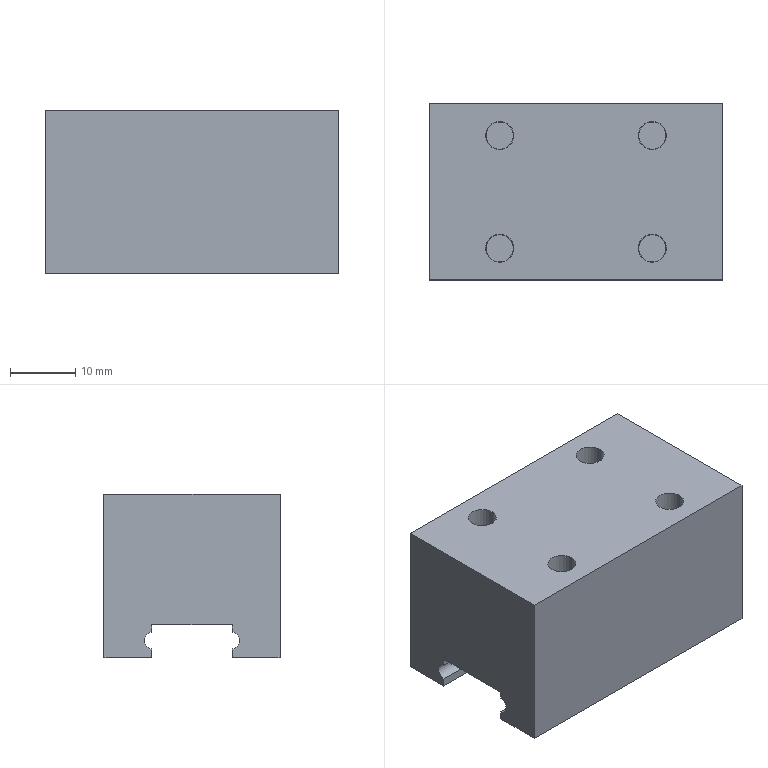Part | SolidWorks | features BaseBody 1 | 1 solid | 38 faces | box 45 x 27 x 25 mm | volume 26500 mm3 | plane 20 | cylinder 18 | commonest cylinder face diameters 4.2 x8 4.3 x8 2.6 x2
STEP:
#1=CARTESIAN_POINT('',(9.55,8.64,21.8));
#2=VERTEX_POINT('',#1);
#3=CARTESIAN_POINT('',(13.85,8.64,21.8));
#4=VERTEX_POINT('',#3);
#5=CARTESIAN_POINT('',(11.7,8.64,21.8));
#6=DIRECTION('',(0.,0.,1.));
#7=DIRECTION('',(1.,0.,0.));
#8=AXIS2_PLACEMENT_3D('',#5,#6,#7);
#9=CIRCLE('',#8,2.15);
#10=EDGE_CURVE('',#2,#4,#9,.T.);
#11=ORIENTED_EDGE('',*,*,#10,.F.);
#12=CARTESIAN_POINT('',(9.55,8.64,28.));
#13=VERTEX_POINT('',#12);
#14=CARTESIAN_POINT('',(9.55,8.64,21.8));
#15=DIRECTION('',(0.,0.,1.));
#16=VECTOR('',#15,1000.);
#17=LINE('',#14,#16);
#18=EDGE_CURVE('',#2,#13,#17,.T.);
#19=ORIENTED_EDGE('',*,*,#18,.T.);
#20=CARTESIAN_POINT('',(13.85,8.64,28.));
#21=VERTEX_POINT('',#20);
#22=CARTESIAN_POINT('',(11.7,8.64,28.));
#23=DIRECTION('',(0.,0.,-1.));
#24=DIRECTION('',(1.,0.,0.));
#25=AXIS2_PLACEMENT_3D('',#22,#23,#24);
#26=CIRCLE('',#25,2.15);
#27=EDGE_CURVE('',#21,#13,#26,.T.);
#28=ORIENTED_EDGE('',*,*,#27,.F.);
#29=CARTESIAN_POINT('',(13.85,8.64,21.8));
#30=DIRECTION('',(0.,0.,1.));
#31=VECTOR('',#30,1000.);
#32=LINE('',#29,#31);
#33=EDGE_CURVE('',#4,#21,#32,.T.);
#34=ORIENTED_EDGE('',*,*,#33,.F.);
#35=EDGE_LOOP('',(#11,#19,#28,#34));
#36=FACE_OUTER_BOUND('',#35,.T.);
#37=CARTESIAN_POINT('',(11.7,8.64,21.8));
#38=DIRECTION('',(0.,0.,1.));
#39=DIRECTION('',(1.,0.,0.));
#40=AXIS2_PLACEMENT_3D('',#37,#38,#39);
#41=CYLINDRICAL_SURFACE('',#40,2.15);
#42=ADVANCED_FACE('',(#36),#41,.F.);
#43=CARTESIAN_POINT('',(-13.85,8.64,21.8));
#44=VERTEX_POINT('',#43);
#45=CARTESIAN_POINT('',(-9.55,8.64,21.8));
#46=VERTEX_POINT('',#45);
#47=CARTESIAN_POINT('',(-11.7,8.64,21.8));
#48=DIRECTION('',(0.,0.,1.));
#49=DIRECTION('',(1.,0.,0.));
#50=AXIS2_PLACEMENT_3D('',#47,#48,#49);
#51=CIRCLE('',#50,2.15);
#52=EDGE_CURVE('',#44,#46,#51,.T.);
#53=ORIENTED_EDGE('',*,*,#52,.F.);
#54=CARTESIAN_POINT('',(-13.85,8.64,28.));
#55=VERTEX_POINT('',#54);
#56=CARTESIAN_POINT('',(-13.85,8.64,21.8));
#57=DIRECTION('',(0.,0.,1.));
#58=VECTOR('',#57,1000.);
#59=LINE('',#56,#58);
#60=EDGE_CURVE('',#44,#55,#59,.T.);
#61=ORIENTED_EDGE('',*,*,#60,.T.);
#62=CARTESIAN_POINT('',(-9.55,8.64,28.));
#63=VERTEX_POINT('',#62);
#64=CARTESIAN_POINT('',(-11.7,8.64,28.));
#65=DIRECTION('',(0.,0.,-1.));
#66=DIRECTION('',(1.,0.,0.));
#67=AXIS2_PLACEMENT_3D('',#64,#65,#66);
#68=CIRCLE('',#67,2.15);
#69=EDGE_CURVE('',#63,#55,#68,.T.);
#70=ORIENTED_EDGE('',*,*,#69,.F.);
#71=CARTESIAN_POINT('',(-9.55,8.64,21.8));
#72=DIRECTION('',(0.,0.,1.));
#73=VECTOR('',#72,1000.);
#74=LINE('',#71,#73);
#75=EDGE_CURVE('',#46,#63,#74,.T.);
#76=ORIENTED_EDGE('',*,*,#75,.F.);
#77=EDGE_LOOP('',(#53,#61,#70,#76));
#78=FACE_OUTER_BOUND('',#77,.T.);
#79=CARTESIAN_POINT('',(-11.7,8.64,21.8));
#80=DIRECTION('',(0.,0.,1.));
#81=DIRECTION('',(1.,0.,0.));
#82=AXIS2_PLACEMENT_3D('',#79,#80,#81);
#83=CYLINDRICAL_SURFACE('',#82,2.15);
#84=ADVANCED_FACE('',(#78),#83,.F.);
#85=CARTESIAN_POINT('',(9.55,-8.64,21.8));
#86=VERTEX_POINT('',#85);
#87=CARTESIAN_POINT('',(13.85,-8.64,21.8));
#88=VERTEX_POINT('',#87);
#89=CARTESIAN_POINT('',(11.7,-8.64,21.8));
#90=DIRECTION('',(0.,0.,1.));
#91=DIRECTION('',(1.,0.,0.));
#92=AXIS2_PLACEMENT_3D('',#89,#90,#91);
#93=CIRCLE('',#92,2.15);
#94=EDGE_CURVE('',#86,#88,#93,.T.);
#95=ORIENTED_EDGE('',*,*,#94,.F.);
#96=CARTESIAN_POINT('',(9.55,-8.64,28.));
#97=VERTEX_POINT('',#96);
#98=CARTESIAN_POINT('',(9.55,-8.64,21.8));
#99=DIRECTION('',(0.,0.,1.));
#100=VECTOR('',#99,1000.);
#101=LINE('',#98,#100);
#102=EDGE_CURVE('',#86,#97,#101,.T.);
#103=ORIENTED_EDGE('',*,*,#102,.T.);
#104=CARTESIAN_POINT('',(13.85,-8.64,28.));
#105=VERTEX_POINT('',#104);
#106=CARTESIAN_POINT('',(11.7,-8.64,28.));
#107=DIRECTION('',(0.,0.,-1.));
#108=DIRECTION('',(1.,0.,0.));
#109=AXIS2_PLACEMENT_3D('',#106,#107,#108);
#110=CIRCLE('',#109,2.15);
#111=EDGE_CURVE('',#105,#97,#110,.T.);
#112=ORIENTED_EDGE('',*,*,#111,.F.);
#113=CARTESIAN_POINT('',(13.85,-8.64,21.8));
#114=DIRECTION('',(0.,0.,1.));
#115=VECTOR('',#114,1000.);
#116=LINE('',#113,#115);
#117=EDGE_CURVE('',#88,#105,#116,.T.);
#118=ORIENTED_EDGE('',*,*,#117,.F.);
#119=EDGE_LOOP('',(#95,#103,#112,#118));
#120=FACE_OUTER_BOUND('',#119,.T.);
#121=CARTESIAN_POINT('',(11.7,-8.64,21.8));
#122=DIRECTION('',(0.,0.,1.));
#123=DIRECTION('',(1.,0.,0.));
#124=AXIS2_PLACEMENT_3D('',#121,#122,#123);
#125=CYLINDRICAL_SURFACE('',#124,2.15);
#126=ADVANCED_FACE('',(#120),#125,.F.);
#127=CARTESIAN_POINT('',(-13.85,-8.64,21.8));
#128=VERTEX_POINT('',#127);
#129=CARTESIAN_POINT('',(-9.55,-8.64,21.8));
#130=VERTEX_POINT('',#129);
#131=CARTESIAN_POINT('',(-11.7,-8.64,21.8));
#132=DIRECTION('',(0.,0.,1.));
#133=DIRECTION('',(1.,0.,0.));
#134=AXIS2_PLACEMENT_3D('',#131,#132,#133);
#135=CIRCLE('',#134,2.15);
#136=EDGE_CURVE('',#128,#130,#135,.T.);
#137=ORIENTED_EDGE('',*,*,#136,.F.);
#138=CARTESIAN_POINT('',(-13.85,-8.64,28.));
#139=VERTEX_POINT('',#138);
#140=CARTESIAN_POINT('',(-13.85,-8.64,21.8));
#141=DIRECTION('',(0.,0.,1.));
#142=VECTOR('',#141,1000.);
#143=LINE('',#140,#142);
#144=EDGE_CURVE('',#128,#139,#143,.T.);
#145=ORIENTED_EDGE('',*,*,#144,.T.);
#146=CARTESIAN_POINT('',(-9.55,-8.64,28.));
#147=VERTEX_POINT('',#146);
#148=CARTESIAN_POINT('',(-11.7,-8.64,28.));
#149=DIRECTION('',(0.,0.,-1.));
#150=DIRECTION('',(1.,0.,0.));
#151=AXIS2_PLACEMENT_3D('',#148,#149,#150);
#152=CIRCLE('',#151,2.15);
#153=EDGE_CURVE('',#147,#139,#152,.T.);
#154=ORIENTED_EDGE('',*,*,#153,.F.);
#155=CARTESIAN_POINT('',(-9.55,-8.64,21.8));
#156=DIRECTION('',(0.,0.,1.));
#157=VECTOR('',#156,1000.);
#158=LINE('',#155,#157);
#159=EDGE_CURVE('',#130,#147,#158,.T.);
#160=ORIENTED_EDGE('',*,*,#159,.F.);
#161=EDGE_LOOP('',(#137,#145,#154,#160));
#162=FACE_OUTER_BOUND('',#161,.T.);
#163=CARTESIAN_POINT('',(-11.7,-8.64,21.8));
#164=DIRECTION('',(0.,0.,1.));
#165=DIRECTION('',(1.,0.,0.));
#166=AXIS2_PLACEMENT_3D('',#163,#164,#165);
#167=CYLINDRICAL_SURFACE('',#166,2.15);
#168=ADVANCED_FACE('',(#162),#167,.F.);
#169=CARTESIAN_POINT('',(9.6,8.64,12.));
#170=VERTEX_POINT('',#169);
#171=CARTESIAN_POINT('',(13.8,8.64,12.));
#172=VERTEX_POINT('',#171);
#173=CARTESIAN_POINT('',(11.7,8.64,12.));
#174=DIRECTION('',(0.,0.,1.));
#175=DIRECTION('',(1.,0.,0.));
#176=AXIS2_PLACEMENT_3D('',#173,#174,#175);
#177=CIRCLE('',#176,2.1);
#178=EDGE_CURVE('',#170,#172,#177,.T.);
#179=ORIENTED_EDGE('',*,*,#178,.F.);
#180=CARTESIAN_POINT('',(9.6,8.64,21.8));
#181=VERTEX_POINT('',#180);
#182=CARTESIAN_POINT('',(9.6,8.64,12.));
#183=DIRECTION('',(0.,0.,1.));
#184=VECTOR('',#183,1000.);
#185=LINE('',#182,#184);
#186=EDGE_CURVE('',#170,#181,#185,.T.);
#187=ORIENTED_EDGE('',*,*,#186,.T.);
#188=CARTESIAN_POINT('',(13.8,8.64,21.8));
#189=VERTEX_POINT('',#188);
#190=CARTESIAN_POINT('',(11.7,8.64,21.8));
#191=DIRECTION('',(0.,0.,-1.));
#192=DIRECTION('',(1.,0.,0.));
#193=AXIS2_PLACEMENT_3D('',#190,#191,#192);
#194=CIRCLE('',#193,2.1);
#195=EDGE_CURVE('',#189,#181,#194,.T.);
#196=ORIENTED_EDGE('',*,*,#195,.F.);
#197=CARTESIAN_POINT('',(13.8,8.64,12.));
#198=DIRECTION('',(0.,0.,1.));
#199=VECTOR('',#198,1000.);
#200=LINE('',#197,#199);
#201=EDGE_CURVE('',#172,#189,#200,.T.);
#202=ORIENTED_EDGE('',*,*,#201,.F.);
#203=EDGE_LOOP('',(#179,#187,#196,#202));
#204=FACE_OUTER_BOUND('',#203,.T.);
#205=CARTESIAN_POINT('',(11.7,8.64,12.));
#206=DIRECTION('',(0.,0.,1.));
#207=DIRECTION('',(1.,0.,0.));
#208=AXIS2_PLACEMENT_3D('',#205,#206,#207);
#209=CYLINDRICAL_SURFACE('',#208,2.1);
#210=ADVANCED_FACE('',(#204),#209,.F.);
#211=CARTESIAN_POINT('',(-13.8,8.64,12.));
#212=VERTEX_POINT('',#211);
#213=CARTESIAN_POINT('',(-9.6,8.64,12.));
#214=VERTEX_POINT('',#213);
#215=CARTESIAN_POINT('',(-11.7,8.64,12.));
#216=DIRECTION('',(0.,0.,1.));
#217=DIRECTION('',(1.,0.,0.));
#218=AXIS2_PLACEMENT_3D('',#215,#216,#217);
#219=CIRCLE('',#218,2.1);
#220=EDGE_CURVE('',#212,#214,#219,.T.);
#221=ORIENTED_EDGE('',*,*,#220,.F.);
#222=CARTESIAN_POINT('',(-13.8,8.64,21.8));
#223=VERTEX_POINT('',#222);
#224=CARTESIAN_POINT('',(-13.8,8.64,12.));
#225=DIRECTION('',(0.,0.,1.));
#226=VECTOR('',#225,1000.);
#227=LINE('',#224,#226);
#228=EDGE_CURVE('',#212,#223,#227,.T.);
#229=ORIENTED_EDGE('',*,*,#228,.T.);
#230=CARTESIAN_POINT('',(-9.6,8.64,21.8));
#231=VERTEX_POINT('',#230);
#232=CARTESIAN_POINT('',(-11.7,8.64,21.8));
#233=DIRECTION('',(0.,0.,-1.));
#234=DIRECTION('',(1.,0.,0.));
#235=AXIS2_PLACEMENT_3D('',#232,#233,#234);
#236=CIRCLE('',#235,2.1);
#237=EDGE_CURVE('',#231,#223,#236,.T.);
#238=ORIENTED_EDGE('',*,*,#237,.F.);
#239=CARTESIAN_POINT('',(-9.6,8.64,12.));
#240=DIRECTION('',(0.,0.,1.));
#241=VECTOR('',#240,1000.);
#242=LINE('',#239,#241);
#243=EDGE_CURVE('',#214,#231,#242,.T.);
#244=ORIENTED_EDGE('',*,*,#243,.F.);
#245=EDGE_LOOP('',(#221,#229,#238,#244));
#246=FACE_OUTER_BOUND('',#245,.T.);
#247=CARTESIAN_POINT('',(-11.7,8.64,12.));
#248=DIRECTION('',(0.,0.,1.));
#249=DIRECTION('',(1.,0.,0.));
#250=AXIS2_PLACEMENT_3D('',#247,#248,#249);
#251=CYLINDRICAL_SURFACE('',#250,2.1);
#252=ADVANCED_FACE('',(#246),#251,.F.);
#253=CARTESIAN_POINT('',(9.6,-8.64,12.));
#254=VERTEX_POINT('',#253);
#255=CARTESIAN_POINT('',(13.8,-8.64,12.));
#256=VERTEX_POINT('',#255);
#257=CARTESIAN_POINT('',(11.7,-8.64,12.));
#258=DIRECTION('',(0.,0.,1.));
#259=DIRECTION('',(1.,0.,0.));
#260=AXIS2_PLACEMENT_3D('',#257,#258,#259);
#261=CIRCLE('',#260,2.1);
#262=EDGE_CURVE('',#254,#256,#261,.T.);
#263=ORIENTED_EDGE('',*,*,#262,.F.);
#264=CARTESIAN_POINT('',(9.6,-8.64,21.8));
#265=VERTEX_POINT('',#264);
#266=CARTESIAN_POINT('',(9.6,-8.64,12.));
#267=DIRECTION('',(0.,0.,1.));
#268=VECTOR('',#267,1000.);
#269=LINE('',#266,#268);
#270=EDGE_CURVE('',#254,#265,#269,.T.);
#271=ORIENTED_EDGE('',*,*,#270,.T.);
#272=CARTESIAN_POINT('',(13.8,-8.64,21.8));
#273=VERTEX_POINT('',#272);
#274=CARTESIAN_POINT('',(11.7,-8.64,21.8));
#275=DIRECTION('',(0.,0.,-1.));
#276=DIRECTION('',(1.,0.,0.));
#277=AXIS2_PLACEMENT_3D('',#274,#275,#276);
#278=CIRCLE('',#277,2.1);
#279=EDGE_CURVE('',#273,#265,#278,.T.);
#280=ORIENTED_EDGE('',*,*,#279,.F.);
#281=CARTESIAN_POINT('',(13.8,-8.64,12.));
#282=DIRECTION('',(0.,0.,1.));
#283=VECTOR('',#282,1000.);
#284=LINE('',#281,#283);
#285=EDGE_CURVE('',#256,#273,#284,.T.);
#286=ORIENTED_EDGE('',*,*,#285,.F.);
#287=EDGE_LOOP('',(#263,#271,#280,#286));
#288=FACE_OUTER_BOUND('',#287,.T.);
#289=CARTESIAN_POINT('',(11.7,-8.64,12.));
#290=DIRECTION('',(0.,0.,1.));
#291=DIRECTION('',(1.,0.,0.));
#292=AXIS2_PLACEMENT_3D('',#289,#290,#291);
#293=CYLINDRICAL_SURFACE('',#292,2.1);
#294=ADVANCED_FACE('',(#288),#293,.F.);
#295=CARTESIAN_POINT('',(-13.8,-8.64,12.));
#296=VERTEX_POINT('',#295);
#297=CARTESIAN_POINT('',(-9.6,-8.64,12.));
#298=VERTEX_POINT('',#297);
#299=CARTESIAN_POINT('',(-11.7,-8.64,12.));
#300=DIRECTION('',(0.,0.,1.));
#301=DIRECTION('',(1.,0.,0.));
#302=AXIS2_PLACEMENT_3D('',#299,#300,#301);
#303=CIRCLE('',#302,2.1);
#304=EDGE_CURVE('',#296,#298,#303,.T.);
#305=ORIENTED_EDGE('',*,*,#304,.F.);
#306=CARTESIAN_POINT('',(-13.8,-8.64,21.8));
#307=VERTEX_POINT('',#306);
#308=CARTESIAN_POINT('',(-13.8,-8.64,12.));
#309=DIRECTION('',(0.,0.,1.));
#310=VECTOR('',#309,1000.);
#311=LINE('',#308,#310);
#312=EDGE_CURVE('',#296,#307,#311,.T.);
#313=ORIENTED_EDGE('',*,*,#312,.T.);
#314=CARTESIAN_POINT('',(-9.6,-8.64,21.8));
#315=VERTEX_POINT('',#314);
#316=CARTESIAN_POINT('',(-11.7,-8.64,21.8));
#317=DIRECTION('',(0.,0.,-1.));
#318=DIRECTION('',(1.,0.,0.));
#319=AXIS2_PLACEMENT_3D('',#316,#317,#318);
#320=CIRCLE('',#319,2.1);
#321=EDGE_CURVE('',#315,#307,#320,.T.);
#322=ORIENTED_EDGE('',*,*,#321,.F.);
#323=CARTESIAN_POINT('',(-9.6,-8.64,12.));
#324=DIRECTION('',(0.,0.,1.));
#325=VECTOR('',#324,1000.);
#326=LINE('',#323,#325);
#327=EDGE_CURVE('',#298,#315,#326,.T.);
#328=ORIENTED_EDGE('',*,*,#327,.F.);
#329=EDGE_LOOP('',(#305,#313,#322,#328));
#330=FACE_OUTER_BOUND('',#329,.T.);
#331=CARTESIAN_POINT('',(-11.7,-8.64,12.));
#332=DIRECTION('',(0.,0.,1.));
#333=DIRECTION('',(1.,0.,0.));
#334=AXIS2_PLACEMENT_3D('',#331,#332,#333);
#335=CYLINDRICAL_SURFACE('',#334,2.1);
#336=ADVANCED_FACE('',(#330),#335,.F.);
#337=ORIENTED_EDGE('',*,*,#27,.T.);
#338=CARTESIAN_POINT('',(11.7,8.64,28.));
#339=DIRECTION('',(0.,0.,-1.));
#340=DIRECTION('',(1.,0.,0.));
#341=AXIS2_PLACEMENT_3D('',#338,#339,#340);
#342=CIRCLE('',#341,2.15);
#343=EDGE_CURVE('',#13,#21,#342,.T.);
#344=ORIENTED_EDGE('',*,*,#343,.T.);
#345=EDGE_LOOP('',(#337,#344));
#346=FACE_BOUND('',#345,.T.);
#347=ORIENTED_EDGE('',*,*,#69,.T.);
#348=CARTESIAN_POINT('',(-11.7,8.64,28.));
#349=DIRECTION('',(0.,0.,-1.));
#350=DIRECTION('',(1.,0.,0.));
#351=AXIS2_PLACEMENT_3D('',#348,#349,#350);
#352=CIRCLE('',#351,2.15);
#353=EDGE_CURVE('',#55,#63,#352,.T.);
#354=ORIENTED_EDGE('',*,*,#353,.T.);
#355=EDGE_LOOP('',(#347,#354));
#356=FACE_BOUND('',#355,.T.);
#357=ORIENTED_EDGE('',*,*,#111,.T.);
#358=CARTESIAN_POINT('',(11.7,-8.64,28.));
#359=DIRECTION('',(0.,0.,-1.));
#360=DIRECTION('',(1.,0.,0.));
#361=AXIS2_PLACEMENT_3D('',#358,#359,#360);
#362=CIRCLE('',#361,2.15);
#363=EDGE_CURVE('',#97,#105,#362,.T.);
#364=ORIENTED_EDGE('',*,*,#363,.T.);
#365=EDGE_LOOP('',(#357,#364));
#366=FACE_BOUND('',#365,.T.);
#367=ORIENTED_EDGE('',*,*,#153,.T.);
#368=CARTESIAN_POINT('',(-11.7,-8.64,28.));
#369=DIRECTION('',(0.,0.,-1.));
#370=DIRECTION('',(1.,0.,0.));
#371=AXIS2_PLACEMENT_3D('',#368,#369,#370);
#372=CIRCLE('',#371,2.15);
#373=EDGE_CURVE('',#139,#147,#372,.T.);
#374=ORIENTED_EDGE('',*,*,#373,.T.);
#375=EDGE_LOOP('',(#367,#374));
#376=FACE_BOUND('',#375,.T.);
#377=CARTESIAN_POINT('',(22.5,-13.5,28.));
#378=VERTEX_POINT('',#377);
#379=CARTESIAN_POINT('',(22.5,13.5,28.));
#380=VERTEX_POINT('',#379);
#381=CARTESIAN_POINT('',(22.5,-13.5,28.));
#382=DIRECTION('',(0.,1.,0.));
#383=VECTOR('',#382,1000.);
#384=LINE('',#381,#383);
#385=EDGE_CURVE('',#378,#380,#384,.T.);
#386=ORIENTED_EDGE('',*,*,#385,.T.);
#387=CARTESIAN_POINT('',(-22.5,13.5,28.));
#388=VERTEX_POINT('',#387);
#389=CARTESIAN_POINT('',(-22.5,13.5,28.));
#390=DIRECTION('',(-1.,0.,0.));
#391=VECTOR('',#390,1000.);
#392=LINE('',#389,#391);
#393=EDGE_CURVE('',#380,#388,#392,.T.);
#394=ORIENTED_EDGE('',*,*,#393,.T.);
#395=CARTESIAN_POINT('',(-22.5,-13.5,28.));
#396=VERTEX_POINT('',#395);
#397=CARTESIAN_POINT('',(-22.5,-13.5,28.));
#398=DIRECTION('',(0.,-1.,0.));
#399=VECTOR('',#398,1000.);
#400=LINE('',#397,#399);
#401=EDGE_CURVE('',#388,#396,#400,.T.);
#402=ORIENTED_EDGE('',*,*,#401,.T.);
#403=CARTESIAN_POINT('',(-22.5,-13.5,28.));
#404=DIRECTION('',(1.,0.,0.));
#405=VECTOR('',#404,1000.);
#406=LINE('',#403,#405);
#407=EDGE_CURVE('',#396,#378,#406,.T.);
#408=ORIENTED_EDGE('',*,*,#407,.T.);
#409=EDGE_LOOP('',(#386,#394,#402,#408));
#410=FACE_OUTER_BOUND('',#409,.T.);
#411=CARTESIAN_POINT('',(-22.5,-13.5,28.));
#412=DIRECTION('',(0.,0.,1.));
#413=DIRECTION('',(1.,0.,0.));
#414=AXIS2_PLACEMENT_3D('',#411,#412,#413);
#415=PLANE('',#414);
#416=ADVANCED_FACE('',(#346,#356,#366,#376,#410),#415,.T.);
#417=ORIENTED_EDGE('',*,*,#18,.F.);
#418=CARTESIAN_POINT('',(11.7,8.64,21.8));
#419=DIRECTION('',(0.,0.,1.));
#420=DIRECTION('',(1.,0.,0.));
#421=AXIS2_PLACEMENT_3D('',#418,#419,#420);
#422=CIRCLE('',#421,2.15);
#423=EDGE_CURVE('',#4,#2,#422,.T.);
#424=ORIENTED_EDGE('',*,*,#423,.F.);
#425=ORIENTED_EDGE('',*,*,#33,.T.);
#426=ORIENTED_EDGE('',*,*,#343,.F.);
#427=EDGE_LOOP('',(#417,#424,#425,#426));
#428=FACE_OUTER_BOUND('',#427,.T.);
#429=CARTESIAN_POINT('',(11.7,8.64,21.8));
#430=DIRECTION('',(0.,0.,1.));
#431=DIRECTION('',(1.,0.,0.));
#432=AXIS2_PLACEMENT_3D('',#429,#430,#431);
#433=CYLINDRICAL_SURFACE('',#432,2.15);
#434=ADVANCED_FACE('',(#428),#433,.F.);
#435=ORIENTED_EDGE('',*,*,#60,.F.);
#436=CARTESIAN_POINT('',(-11.7,8.64,21.8));
#437=DIRECTION('',(0.,0.,1.));
#438=DIRECTION('',(1.,0.,0.));
#439=AXIS2_PLACEMENT_3D('',#436,#437,#438);
#440=CIRCLE('',#439,2.15);
#441=EDGE_CURVE('',#46,#44,#440,.T.);
#442=ORIENTED_EDGE('',*,*,#441,.F.);
#443=ORIENTED_EDGE('',*,*,#75,.T.);
#444=ORIENTED_EDGE('',*,*,#353,.F.);
#445=EDGE_LOOP('',(#435,#442,#443,#444));
#446=FACE_OUTER_BOUND('',#445,.T.);
#447=CARTESIAN_POINT('',(-11.7,8.64,21.8));
#448=DIRECTION('',(0.,0.,1.));
#449=DIRECTION('',(1.,0.,0.));
#450=AXIS2_PLACEMENT_3D('',#447,#448,#449);
#451=CYLINDRICAL_SURFACE('',#450,2.15);
#452=ADVANCED_FACE('',(#446),#451,.F.);
#453=ORIENTED_EDGE('',*,*,#102,.F.);
#454=CARTESIAN_POINT('',(11.7,-8.64,21.8));
#455=DIRECTION('',(0.,0.,1.));
#456=DIRECTION('',(1.,0.,0.));
#457=AXIS2_PLACEMENT_3D('',#454,#455,#456);
#458=CIRCLE('',#457,2.15);
#459=EDGE_CURVE('',#88,#86,#458,.T.);
#460=ORIENTED_EDGE('',*,*,#459,.F.);
#461=ORIENTED_EDGE('',*,*,#117,.T.);
#462=ORIENTED_EDGE('',*,*,#363,.F.);
#463=EDGE_LOOP('',(#453,#460,#461,#462));
#464=FACE_OUTER_BOUND('',#463,.T.);
#465=CARTESIAN_POINT('',(11.7,-8.64,21.8));
#466=DIRECTION('',(0.,0.,1.));
#467=DIRECTION('',(1.,0.,0.));
#468=AXIS2_PLACEMENT_3D('',#465,#466,#467);
#469=CYLINDRICAL_SURFACE('',#468,2.15);
#470=ADVANCED_FACE('',(#464),#469,.F.);
#471=ORIENTED_EDGE('',*,*,#144,.F.);
#472=CARTESIAN_POINT('',(-11.7,-8.64,21.8));
#473=DIRECTION('',(0.,0.,1.));
#474=DIRECTION('',(1.,0.,0.));
#475=AXIS2_PLACEMENT_3D('',#472,#473,#474);
#476=CIRCLE('',#475,2.15);
#477=EDGE_CURVE('',#130,#128,#476,.T.);
#478=ORIENTED_EDGE('',*,*,#477,.F.);
#479=ORIENTED_EDGE('',*,*,#159,.T.);
#480=ORIENTED_EDGE('',*,*,#373,.F.);
#481=EDGE_LOOP('',(#471,#478,#479,#480));
#482=FACE_OUTER_BOUND('',#481,.T.);
#483=CARTESIAN_POINT('',(-11.7,-8.64,21.8));
#484=DIRECTION('',(0.,0.,1.));
#485=DIRECTION('',(1.,0.,0.));
#486=AXIS2_PLACEMENT_3D('',#483,#484,#485);
#487=CYLINDRICAL_SURFACE('',#486,2.15);
#488=ADVANCED_FACE('',(#482),#487,.F.);
#489=ORIENTED_EDGE('',*,*,#393,.F.);
#490=CARTESIAN_POINT('',(22.5,13.5,3.));
#491=VERTEX_POINT('',#490);
#492=CARTESIAN_POINT('',(22.5,13.5,3.));
#493=DIRECTION('',(0.,0.,-1.));
#494=VECTOR('',#493,1000.);
#495=LINE('',#492,#494);
#496=EDGE_CURVE('',#380,#491,#495,.T.);
#497=ORIENTED_EDGE('',*,*,#496,.T.);
#498=CARTESIAN_POINT('',(-22.5,13.5,3.));
#499=VERTEX_POINT('',#498);
#500=CARTESIAN_POINT('',(-22.5,13.5,3.));
#501=DIRECTION('',(-1.,0.,0.));
#502=VECTOR('',#501,1000.);
#503=LINE('',#500,#502);
#504=EDGE_CURVE('',#491,#499,#503,.T.);
#505=ORIENTED_EDGE('',*,*,#504,.T.);
#506=CARTESIAN_POINT('',(-22.5,13.5,3.));
#507=DIRECTION('',(0.,0.,1.));
#508=VECTOR('',#507,1000.);
#509=LINE('',#506,#508);
#510=EDGE_CURVE('',#499,#388,#509,.T.);
#511=ORIENTED_EDGE('',*,*,#510,.T.);
#512=EDGE_LOOP('',(#489,#497,#505,#511));
#513=FACE_OUTER_BOUND('',#512,.T.);
#514=CARTESIAN_POINT('',(-22.5,13.5,3.));
#515=DIRECTION('',(0.,1.,0.));
#516=DIRECTION('',(0.,0.,1.));
#517=AXIS2_PLACEMENT_3D('',#514,#515,#516);
#518=PLANE('',#517);
#519=ADVANCED_FACE('',(#513),#518,.T.);
#520=CARTESIAN_POINT('',(22.5,6.15,4.309));
#521=VERTEX_POINT('',#520);
#522=CARTESIAN_POINT('',(22.5,6.15,3.));
#523=VERTEX_POINT('',#522);
#524=CARTESIAN_POINT('',(22.5,6.15,-0.3));
#525=DIRECTION('',(0.,0.,-1.));
#526=VECTOR('',#525,1000.);
#527=LINE('',#524,#526);
#528=EDGE_CURVE('',#521,#523,#527,.T.);
#529=ORIENTED_EDGE('',*,*,#528,.T.);
#530=CARTESIAN_POINT('',(22.5,-13.5,3.));
#531=DIRECTION('',(0.,1.,0.));
#532=VECTOR('',#531,1000.);
#533=LINE('',#530,#532);
#534=EDGE_CURVE('',#523,#491,#533,.T.);
#535=ORIENTED_EDGE('',*,*,#534,.T.);
#536=ORIENTED_EDGE('',*,*,#496,.F.);
#537=ORIENTED_EDGE('',*,*,#385,.F.);
#538=CARTESIAN_POINT('',(22.5,-13.5,3.));
#539=VERTEX_POINT('',#538);
#540=CARTESIAN_POINT('',(22.5,-13.5,3.));
#541=DIRECTION('',(0.,0.,-1.));
#542=VECTOR('',#541,1000.);
#543=LINE('',#540,#542);
#544=EDGE_CURVE('',#378,#539,#543,.T.);
#545=ORIENTED_EDGE('',*,*,#544,.T.);
#546=CARTESIAN_POINT('',(22.5,-6.15,3.));
#547=VERTEX_POINT('',#546);
#548=CARTESIAN_POINT('',(22.5,-13.5,3.));
#549=DIRECTION('',(0.,1.,0.));
#550=VECTOR('',#549,1000.);
#551=LINE('',#548,#550);
#552=EDGE_CURVE('',#539,#547,#551,.T.);
#553=ORIENTED_EDGE('',*,*,#552,.T.);
#554=CARTESIAN_POINT('',(22.5,-6.15,4.309));
#555=VERTEX_POINT('',#554);
#556=CARTESIAN_POINT('',(22.5,-6.15,-0.3));
#557=DIRECTION('',(0.,0.,-1.));
#558=VECTOR('',#557,1000.);
#559=LINE('',#556,#558);
#560=EDGE_CURVE('',#555,#547,#559,.T.);
#561=ORIENTED_EDGE('',*,*,#560,.F.);
#562=CARTESIAN_POINT('',(22.5,-6.15,6.891));
#563=VERTEX_POINT('',#562);
#564=CARTESIAN_POINT('',(22.5,-6.,5.6));
#565=DIRECTION('',(-1.,0.,0.));
#566=DIRECTION('',(0.,0.,-1.));
#567=AXIS2_PLACEMENT_3D('',#564,#565,#566);
#568=CIRCLE('',#567,1.3);
#569=EDGE_CURVE('',#555,#563,#568,.T.);
#570=ORIENTED_EDGE('',*,*,#569,.T.);
#571=CARTESIAN_POINT('',(22.5,-6.15,8.));
#572=VERTEX_POINT('',#571);
#573=CARTESIAN_POINT('',(22.5,-6.15,-0.3));
#574=DIRECTION('',(0.,0.,-1.));
#575=VECTOR('',#574,1000.);
#576=LINE('',#573,#575);
#577=EDGE_CURVE('',#572,#563,#576,.T.);
#578=ORIENTED_EDGE('',*,*,#577,.F.);
#579=CARTESIAN_POINT('',(22.5,6.15,8.));
#580=VERTEX_POINT('',#579);
#581=CARTESIAN_POINT('',(22.5,-13.5,8.));
#582=DIRECTION('',(0.,1.,0.));
#583=VECTOR('',#582,1000.);
#584=LINE('',#581,#583);
#585=EDGE_CURVE('',#572,#580,#584,.T.);
#586=ORIENTED_EDGE('',*,*,#585,.T.);
#587=CARTESIAN_POINT('',(22.5,6.15,6.891));
#588=VERTEX_POINT('',#587);
#589=CARTESIAN_POINT('',(22.5,6.15,-0.3));
#590=DIRECTION('',(0.,0.,-1.));
#591=VECTOR('',#590,1000.);
#592=LINE('',#589,#591);
#593=EDGE_CURVE('',#580,#588,#592,.T.);
#594=ORIENTED_EDGE('',*,*,#593,.T.);
#595=CARTESIAN_POINT('',(22.5,6.,5.6));
#596=DIRECTION('',(-1.,0.,0.));
#597=DIRECTION('',(0.,0.,-1.));
#598=AXIS2_PLACEMENT_3D('',#595,#596,#597);
#599=CIRCLE('',#598,1.3);
#600=EDGE_CURVE('',#588,#521,#599,.T.);
#601=ORIENTED_EDGE('',*,*,#600,.T.);
#602=EDGE_LOOP('',(#529,#535,#536,#537,#545,#553,#561,#570,#578,#586,#594,#601));
#603=FACE_OUTER_BOUND('',#602,.T.);
#604=CARTESIAN_POINT('',(22.5,-13.5,3.));
#605=DIRECTION('',(1.,0.,0.));
#606=DIRECTION('',(0.,0.,-1.));
#607=AXIS2_PLACEMENT_3D('',#604,#605,#606);
#608=PLANE('',#607);
#609=ADVANCED_FACE('',(#603),#608,.T.);
#610=ORIENTED_EDGE('',*,*,#407,.F.);
#611=CARTESIAN_POINT('',(-22.5,-13.5,3.));
#612=VERTEX_POINT('',#611);
#613=CARTESIAN_POINT('',(-22.5,-13.5,3.));
#614=DIRECTION('',(0.,0.,1.));
#615=VECTOR('',#614,1000.);
#616=LINE('',#613,#615);
#617=EDGE_CURVE('',#612,#396,#616,.T.);
#618=ORIENTED_EDGE('',*,*,#617,.F.);
#619=CARTESIAN_POINT('',(-22.5,-13.5,3.));
#620=DIRECTION('',(-1.,0.,0.));
#621=VECTOR('',#620,1000.);
#622=LINE('',#619,#621);
#623=EDGE_CURVE('',#539,#612,#622,.T.);
#624=ORIENTED_EDGE('',*,*,#623,.F.);
#625=ORIENTED_EDGE('',*,*,#544,.F.);
#626=EDGE_LOOP('',(#610,#618,#624,#625));
#627=FACE_OUTER_BOUND('',#626,.T.);
#628=CARTESIAN_POINT('',(-22.5,-13.5,3.));
#629=DIRECTION('',(0.,1.,0.));
#630=DIRECTION('',(0.,0.,1.));
#631=AXIS2_PLACEMENT_3D('',#628,#629,#630);
#632=PLANE('',#631);
#633=ADVANCED_FACE('',(#627),#632,.F.);
#634=CARTESIAN_POINT('',(-22.5,6.15,3.));
#635=VERTEX_POINT('',#634);
#636=CARTESIAN_POINT('',(-22.5,6.15,4.309));
#637=VERTEX_POINT('',#636);
#638=CARTESIAN_POINT('',(-22.5,6.15,-0.3));
#639=DIRECTION('',(0.,0.,1.));
#640=VECTOR('',#639,1000.);
#641=LINE('',#638,#640);
#642=EDGE_CURVE('',#635,#637,#641,.T.);
#643=ORIENTED_EDGE('',*,*,#642,.T.);
#644=CARTESIAN_POINT('',(-22.5,6.15,6.891));
#645=VERTEX_POINT('',#644);
#646=CARTESIAN_POINT('',(-22.5,6.,5.6));
#647=DIRECTION('',(-1.,0.,0.));
#648=DIRECTION('',(0.,0.,-1.));
#649=AXIS2_PLACEMENT_3D('',#646,#647,#648);
#650=CIRCLE('',#649,1.3);
#651=EDGE_CURVE('',#645,#637,#650,.T.);
#652=ORIENTED_EDGE('',*,*,#651,.F.);
#653=CARTESIAN_POINT('',(-22.5,6.15,8.));
#654=VERTEX_POINT('',#653);
#655=CARTESIAN_POINT('',(-22.5,6.15,-0.3));
#656=DIRECTION('',(0.,0.,1.));
#657=VECTOR('',#656,1000.);
#658=LINE('',#655,#657);
#659=EDGE_CURVE('',#645,#654,#658,.T.);
#660=ORIENTED_EDGE('',*,*,#659,.T.);
#661=CARTESIAN_POINT('',(-22.5,-6.15,8.));
#662=VERTEX_POINT('',#661);
#663=CARTESIAN_POINT('',(-22.5,-13.5,8.));
#664=DIRECTION('',(0.,1.,0.));
#665=VECTOR('',#664,1000.);
#666=LINE('',#663,#665);
#667=EDGE_CURVE('',#662,#654,#666,.T.);
#668=ORIENTED_EDGE('',*,*,#667,.F.);
#669=CARTESIAN_POINT('',(-22.5,-6.15,6.891));
#670=VERTEX_POINT('',#669);
#671=CARTESIAN_POINT('',(-22.5,-6.15,-0.3));
#672=DIRECTION('',(0.,0.,1.));
#673=VECTOR('',#672,1000.);
#674=LINE('',#671,#673);
#675=EDGE_CURVE('',#670,#662,#674,.T.);
#676=ORIENTED_EDGE('',*,*,#675,.F.);
#677=CARTESIAN_POINT('',(-22.5,-6.15,4.309));
#678=VERTEX_POINT('',#677);
#679=CARTESIAN_POINT('',(-22.5,-6.,5.6));
#680=DIRECTION('',(-1.,0.,0.));
#681=DIRECTION('',(0.,0.,-1.));
#682=AXIS2_PLACEMENT_3D('',#679,#680,#681);
#683=CIRCLE('',#682,1.3);
#684=EDGE_CURVE('',#678,#670,#683,.T.);
#685=ORIENTED_EDGE('',*,*,#684,.F.);
#686=CARTESIAN_POINT('',(-22.5,-6.15,3.));
#687=VERTEX_POINT('',#686);
#688=CARTESIAN_POINT('',(-22.5,-6.15,-0.3));
#689=DIRECTION('',(0.,0.,1.));
#690=VECTOR('',#689,1000.);
#691=LINE('',#688,#690);
#692=EDGE_CURVE('',#687,#678,#691,.T.);
#693=ORIENTED_EDGE('',*,*,#692,.F.);
#694=CARTESIAN_POINT('',(-22.5,-13.5,3.));
#695=DIRECTION('',(0.,1.,0.));
#696=VECTOR('',#695,1000.);
#697=LINE('',#694,#696);
#698=EDGE_CURVE('',#612,#687,#697,.T.);
#699=ORIENTED_EDGE('',*,*,#698,.F.);
#700=ORIENTED_EDGE('',*,*,#617,.T.);
#701=ORIENTED_EDGE('',*,*,#401,.F.);
#702=ORIENTED_EDGE('',*,*,#510,.F.);
#703=CARTESIAN_POINT('',(-22.5,-13.5,3.));
#704=DIRECTION('',(0.,1.,0.));
#705=VECTOR('',#704,1000.);
#706=LINE('',#703,#705);
#707=EDGE_CURVE('',#635,#499,#706,.T.);
#708=ORIENTED_EDGE('',*,*,#707,.F.);
#709=EDGE_LOOP('',(#643,#652,#660,#668,#676,#685,#693,#699,#700,#701,#702,#708));
#710=FACE_OUTER_BOUND('',#709,.T.);
#711=CARTESIAN_POINT('',(-22.5,-13.5,3.));
#712=DIRECTION('',(1.,0.,0.));
#713=DIRECTION('',(0.,0.,-1.));
#714=AXIS2_PLACEMENT_3D('',#711,#712,#713);
#715=PLANE('',#714);
#716=ADVANCED_FACE('',(#710),#715,.F.);
#717=ORIENTED_EDGE('',*,*,#195,.T.);
#718=CARTESIAN_POINT('',(11.7,8.64,21.8));
#719=DIRECTION('',(0.,0.,-1.));
#720=DIRECTION('',(1.,0.,0.));
#721=AXIS2_PLACEMENT_3D('',#718,#719,#720);
#722=CIRCLE('',#721,2.1);
#723=EDGE_CURVE('',#181,#189,#722,.T.);
#724=ORIENTED_EDGE('',*,*,#723,.T.);
#725=EDGE_LOOP('',(#717,#724));
#726=FACE_BOUND('',#725,.T.);
#727=ORIENTED_EDGE('',*,*,#423,.T.);
#728=ORIENTED_EDGE('',*,*,#10,.T.);
#729=EDGE_LOOP('',(#727,#728));
#730=FACE_OUTER_BOUND('',#729,.T.);
#731=CARTESIAN_POINT('',(11.7,8.64,21.8));
#732=DIRECTION('',(0.,0.,1.));
#733=DIRECTION('',(1.,0.,0.));
#734=AXIS2_PLACEMENT_3D('',#731,#732,#733);
#735=PLANE('',#734);
#736=ADVANCED_FACE('',(#726,#730),#735,.T.);
#737=ORIENTED_EDGE('',*,*,#237,.T.);
#738=CARTESIAN_POINT('',(-11.7,8.64,21.8));
#739=DIRECTION('',(0.,0.,-1.));
#740=DIRECTION('',(1.,0.,0.));
#741=AXIS2_PLACEMENT_3D('',#738,#739,#740);
#742=CIRCLE('',#741,2.1);
#743=EDGE_CURVE('',#223,#231,#742,.T.);
#744=ORIENTED_EDGE('',*,*,#743,.T.);
#745=EDGE_LOOP('',(#737,#744));
#746=FACE_BOUND('',#745,.T.);
#747=ORIENTED_EDGE('',*,*,#441,.T.);
#748=ORIENTED_EDGE('',*,*,#52,.T.);
#749=EDGE_LOOP('',(#747,#748));
#750=FACE_OUTER_BOUND('',#749,.T.);
#751=CARTESIAN_POINT('',(-11.7,8.64,21.8));
#752=DIRECTION('',(0.,0.,1.));
#753=DIRECTION('',(1.,0.,0.));
#754=AXIS2_PLACEMENT_3D('',#751,#752,#753);
#755=PLANE('',#754);
#756=ADVANCED_FACE('',(#746,#750),#755,.T.);
#757=ORIENTED_EDGE('',*,*,#279,.T.);
#758=CARTESIAN_POINT('',(11.7,-8.64,21.8));
#759=DIRECTION('',(0.,0.,-1.));
#760=DIRECTION('',(1.,0.,0.));
#761=AXIS2_PLACEMENT_3D('',#758,#759,#760);
#762=CIRCLE('',#761,2.1);
#763=EDGE_CURVE('',#265,#273,#762,.T.);
#764=ORIENTED_EDGE('',*,*,#763,.T.);
#765=EDGE_LOOP('',(#757,#764));
#766=FACE_BOUND('',#765,.T.);
#767=ORIENTED_EDGE('',*,*,#459,.T.);
#768=ORIENTED_EDGE('',*,*,#94,.T.);
#769=EDGE_LOOP('',(#767,#768));
#770=FACE_OUTER_BOUND('',#769,.T.);
#771=CARTESIAN_POINT('',(11.7,-8.64,21.8));
#772=DIRECTION('',(0.,0.,1.));
#773=DIRECTION('',(1.,0.,0.));
#774=AXIS2_PLACEMENT_3D('',#771,#772,#773);
#775=PLANE('',#774);
#776=ADVANCED_FACE('',(#766,#770),#775,.T.);
#777=ORIENTED_EDGE('',*,*,#321,.T.);
#778=CARTESIAN_POINT('',(-11.7,-8.64,21.8));
#779=DIRECTION('',(0.,0.,-1.));
#780=DIRECTION('',(1.,0.,0.));
#781=AXIS2_PLACEMENT_3D('',#778,#779,#780);
#782=CIRCLE('',#781,2.1);
#783=EDGE_CURVE('',#307,#315,#782,.T.);
#784=ORIENTED_EDGE('',*,*,#783,.T.);
#785=EDGE_LOOP('',(#777,#784));
#786=FACE_BOUND('',#785,.T.);
#787=ORIENTED_EDGE('',*,*,#477,.T.);
#788=ORIENTED_EDGE('',*,*,#136,.T.);
#789=EDGE_LOOP('',(#787,#788));
#790=FACE_OUTER_BOUND('',#789,.T.);
#791=CARTESIAN_POINT('',(-11.7,-8.64,21.8));
#792=DIRECTION('',(0.,0.,1.));
#793=DIRECTION('',(1.,0.,0.));
#794=AXIS2_PLACEMENT_3D('',#791,#792,#793);
#795=PLANE('',#794);
#796=ADVANCED_FACE('',(#786,#790),#795,.T.);
#797=ORIENTED_EDGE('',*,*,#534,.F.);
#798=CARTESIAN_POINT('',(-22.5,6.15,3.));
#799=DIRECTION('',(1.,0.,0.));
#800=VECTOR('',#799,1000.);
#801=LINE('',#798,#800);
#802=EDGE_CURVE('',#635,#523,#801,.T.);
#803=ORIENTED_EDGE('',*,*,#802,.F.);
#804=ORIENTED_EDGE('',*,*,#707,.T.);
#805=ORIENTED_EDGE('',*,*,#504,.F.);
#806=EDGE_LOOP('',(#797,#803,#804,#805));
#807=FACE_OUTER_BOUND('',#806,.T.);
#808=CARTESIAN_POINT('',(-22.5,-13.5,3.));
#809=DIRECTION('',(0.,0.,1.));
#810=DIRECTION('',(1.,0.,0.));
#811=AXIS2_PLACEMENT_3D('',#808,#809,#810);
#812=PLANE('',#811);
#813=ADVANCED_FACE('',(#807),#812,.F.);
#814=CARTESIAN_POINT('',(-23.5,6.15,6.891));
#815=DIRECTION('',(1.,0.,0.));
#816=VECTOR('',#815,1000.);
#817=LINE('',#814,#816);
#818=EDGE_CURVE('',#645,#588,#817,.T.);
#819=ORIENTED_EDGE('',*,*,#818,.F.);
#820=ORIENTED_EDGE('',*,*,#651,.T.);
#821=CARTESIAN_POINT('',(-23.5,6.15,4.309));
#822=DIRECTION('',(-1.,0.,0.));
#823=VECTOR('',#822,1000.);
#824=LINE('',#821,#823);
#825=EDGE_CURVE('',#521,#637,#824,.T.);
#826=ORIENTED_EDGE('',*,*,#825,.F.);
#827=ORIENTED_EDGE('',*,*,#600,.F.);
#828=EDGE_LOOP('',(#819,#820,#826,#827));
#829=FACE_OUTER_BOUND('',#828,.T.);
#830=CARTESIAN_POINT('',(-23.5,6.,5.6));
#831=DIRECTION('',(1.,0.,0.));
#832=DIRECTION('',(0.,0.,-1.));
#833=AXIS2_PLACEMENT_3D('',#830,#831,#832);
#834=CYLINDRICAL_SURFACE('',#833,1.3);
#835=ADVANCED_FACE('',(#829),#834,.F.);
#836=CARTESIAN_POINT('',(-23.5,-6.15,8.));
#837=DIRECTION('',(1.,0.,0.));
#838=VECTOR('',#837,1000.);
#839=LINE('',#836,#838);
#840=EDGE_CURVE('',#662,#572,#839,.T.);
#841=ORIENTED_EDGE('',*,*,#840,.F.);
#842=ORIENTED_EDGE('',*,*,#667,.T.);
#843=CARTESIAN_POINT('',(-23.5,6.15,8.));
#844=DIRECTION('',(-1.,0.,0.));
#845=VECTOR('',#844,1000.);
#846=LINE('',#843,#845);
#847=EDGE_CURVE('',#580,#654,#846,.T.);
#848=ORIENTED_EDGE('',*,*,#847,.F.);
#849=ORIENTED_EDGE('',*,*,#585,.F.);
#850=EDGE_LOOP('',(#841,#842,#848,#849));
#851=FACE_OUTER_BOUND('',#850,.T.);
#852=CARTESIAN_POINT('',(-23.5,-6.15,8.));
#853=DIRECTION('',(0.,0.,1.));
#854=DIRECTION('',(1.,0.,0.));
#855=AXIS2_PLACEMENT_3D('',#852,#853,#854);
#856=PLANE('',#855);
#857=ADVANCED_FACE('',(#851),#856,.F.);
#858=CARTESIAN_POINT('',(-23.5,-6.15,4.309));
#859=DIRECTION('',(1.,0.,0.));
#860=VECTOR('',#859,1000.);
#861=LINE('',#858,#860);
#862=EDGE_CURVE('',#678,#555,#861,.T.);
#863=ORIENTED_EDGE('',*,*,#862,.F.);
#864=ORIENTED_EDGE('',*,*,#684,.T.);
#865=CARTESIAN_POINT('',(-23.5,-6.15,6.891));
#866=DIRECTION('',(-1.,0.,0.));
#867=VECTOR('',#866,1000.);
#868=LINE('',#865,#867);
#869=EDGE_CURVE('',#563,#670,#868,.T.);
#870=ORIENTED_EDGE('',*,*,#869,.F.);
#871=ORIENTED_EDGE('',*,*,#569,.F.);
#872=EDGE_LOOP('',(#863,#864,#870,#871));
#873=FACE_OUTER_BOUND('',#872,.T.);
#874=CARTESIAN_POINT('',(-23.5,-6.,5.6));
#875=DIRECTION('',(1.,0.,0.));
#876=DIRECTION('',(0.,0.,-1.));
#877=AXIS2_PLACEMENT_3D('',#874,#875,#876);
#878=CYLINDRICAL_SURFACE('',#877,1.3);
#879=ADVANCED_FACE('',(#873),#878,.F.);
#880=ORIENTED_EDGE('',*,*,#552,.F.);
#881=ORIENTED_EDGE('',*,*,#623,.T.);
#882=ORIENTED_EDGE('',*,*,#698,.T.);
#883=CARTESIAN_POINT('',(-22.5,-6.15,3.));
#884=DIRECTION('',(-1.,0.,0.));
#885=VECTOR('',#884,1000.);
#886=LINE('',#883,#885);
#887=EDGE_CURVE('',#547,#687,#886,.T.);
#888=ORIENTED_EDGE('',*,*,#887,.F.);
#889=EDGE_LOOP('',(#880,#881,#882,#888));
#890=FACE_OUTER_BOUND('',#889,.T.);
#891=CARTESIAN_POINT('',(-22.5,-13.5,3.));
#892=DIRECTION('',(0.,0.,1.));
#893=DIRECTION('',(1.,0.,0.));
#894=AXIS2_PLACEMENT_3D('',#891,#892,#893);
#895=PLANE('',#894);
#896=ADVANCED_FACE('',(#890),#895,.F.);
#897=ORIENTED_EDGE('',*,*,#186,.F.);
#898=CARTESIAN_POINT('',(11.7,8.64,12.));
#899=DIRECTION('',(0.,0.,1.));
#900=DIRECTION('',(1.,0.,0.));
#901=AXIS2_PLACEMENT_3D('',#898,#899,#900);
#902=CIRCLE('',#901,2.1);
#903=EDGE_CURVE('',#172,#170,#902,.T.);
#904=ORIENTED_EDGE('',*,*,#903,.F.);
#905=ORIENTED_EDGE('',*,*,#201,.T.);
#906=ORIENTED_EDGE('',*,*,#723,.F.);
#907=EDGE_LOOP('',(#897,#904,#905,#906));
#908=FACE_OUTER_BOUND('',#907,.T.);
#909=CARTESIAN_POINT('',(11.7,8.64,12.));
#910=DIRECTION('',(0.,0.,1.));
#911=DIRECTION('',(1.,0.,0.));
#912=AXIS2_PLACEMENT_3D('',#909,#910,#911);
#913=CYLINDRICAL_SURFACE('',#912,2.1);
#914=ADVANCED_FACE('',(#908),#913,.F.);
#915=ORIENTED_EDGE('',*,*,#228,.F.);
#916=CARTESIAN_POINT('',(-11.7,8.64,12.));
#917=DIRECTION('',(0.,0.,1.));
#918=DIRECTION('',(1.,0.,0.));
#919=AXIS2_PLACEMENT_3D('',#916,#917,#918);
#920=CIRCLE('',#919,2.1);
#921=EDGE_CURVE('',#214,#212,#920,.T.);
#922=ORIENTED_EDGE('',*,*,#921,.F.);
#923=ORIENTED_EDGE('',*,*,#243,.T.);
#924=ORIENTED_EDGE('',*,*,#743,.F.);
#925=EDGE_LOOP('',(#915,#922,#923,#924));
#926=FACE_OUTER_BOUND('',#925,.T.);
#927=CARTESIAN_POINT('',(-11.7,8.64,12.));
#928=DIRECTION('',(0.,0.,1.));
#929=DIRECTION('',(1.,0.,0.));
#930=AXIS2_PLACEMENT_3D('',#927,#928,#929);
#931=CYLINDRICAL_SURFACE('',#930,2.1);
#932=ADVANCED_FACE('',(#926),#931,.F.);
#933=ORIENTED_EDGE('',*,*,#270,.F.);
#934=CARTESIAN_POINT('',(11.7,-8.64,12.));
#935=DIRECTION('',(0.,0.,1.));
#936=DIRECTION('',(1.,0.,0.));
#937=AXIS2_PLACEMENT_3D('',#934,#935,#936);
#938=CIRCLE('',#937,2.1);
#939=EDGE_CURVE('',#256,#254,#938,.T.);
#940=ORIENTED_EDGE('',*,*,#939,.F.);
#941=ORIENTED_EDGE('',*,*,#285,.T.);
#942=ORIENTED_EDGE('',*,*,#763,.F.);
#943=EDGE_LOOP('',(#933,#940,#941,#942));
#944=FACE_OUTER_BOUND('',#943,.T.);
#945=CARTESIAN_POINT('',(11.7,-8.64,12.));
#946=DIRECTION('',(0.,0.,1.));
#947=DIRECTION('',(1.,0.,0.));
#948=AXIS2_PLACEMENT_3D('',#945,#946,#947);
#949=CYLINDRICAL_SURFACE('',#948,2.1);
#950=ADVANCED_FACE('',(#944),#949,.F.);
#951=ORIENTED_EDGE('',*,*,#312,.F.);
#952=CARTESIAN_POINT('',(-11.7,-8.64,12.));
#953=DIRECTION('',(0.,0.,1.));
#954=DIRECTION('',(1.,0.,0.));
#955=AXIS2_PLACEMENT_3D('',#952,#953,#954);
#956=CIRCLE('',#955,2.1);
#957=EDGE_CURVE('',#298,#296,#956,.T.);
#958=ORIENTED_EDGE('',*,*,#957,.F.);
#959=ORIENTED_EDGE('',*,*,#327,.T.);
#960=ORIENTED_EDGE('',*,*,#783,.F.);
#961=EDGE_LOOP('',(#951,#958,#959,#960));
#962=FACE_OUTER_BOUND('',#961,.T.);
#963=CARTESIAN_POINT('',(-11.7,-8.64,12.));
#964=DIRECTION('',(0.,0.,1.));
#965=DIRECTION('',(1.,0.,0.));
#966=AXIS2_PLACEMENT_3D('',#963,#964,#965);
#967=CYLINDRICAL_SURFACE('',#966,2.1);
#968=ADVANCED_FACE('',(#962),#967,.F.);
#969=ORIENTED_EDGE('',*,*,#528,.F.);
#970=ORIENTED_EDGE('',*,*,#825,.T.);
#971=ORIENTED_EDGE('',*,*,#642,.F.);
#972=ORIENTED_EDGE('',*,*,#802,.T.);
#973=EDGE_LOOP('',(#969,#970,#971,#972));
#974=FACE_OUTER_BOUND('',#973,.T.);
#975=CARTESIAN_POINT('',(-23.5,6.15,-0.3));
#976=DIRECTION('',(0.,1.,0.));
#977=DIRECTION('',(0.,0.,1.));
#978=AXIS2_PLACEMENT_3D('',#975,#976,#977);
#979=PLANE('',#978);
#980=ADVANCED_FACE('',(#974),#979,.F.);
#981=ORIENTED_EDGE('',*,*,#593,.F.);
#982=ORIENTED_EDGE('',*,*,#847,.T.);
#983=ORIENTED_EDGE('',*,*,#659,.F.);
#984=ORIENTED_EDGE('',*,*,#818,.T.);
#985=EDGE_LOOP('',(#981,#982,#983,#984));
#986=FACE_OUTER_BOUND('',#985,.T.);
#987=CARTESIAN_POINT('',(-23.5,6.15,-0.3));
#988=DIRECTION('',(0.,1.,0.));
#989=DIRECTION('',(0.,0.,1.));
#990=AXIS2_PLACEMENT_3D('',#987,#988,#989);
#991=PLANE('',#990);
#992=ADVANCED_FACE('',(#986),#991,.F.);
#993=ORIENTED_EDGE('',*,*,#577,.T.);
#994=ORIENTED_EDGE('',*,*,#869,.T.);
#995=ORIENTED_EDGE('',*,*,#675,.T.);
#996=ORIENTED_EDGE('',*,*,#840,.T.);
#997=EDGE_LOOP('',(#993,#994,#995,#996));
#998=FACE_OUTER_BOUND('',#997,.T.);
#999=CARTESIAN_POINT('',(-23.5,-6.15,-0.3));
#1000=DIRECTION('',(0.,1.,0.));
#1001=DIRECTION('',(0.,0.,1.));
#1002=AXIS2_PLACEMENT_3D('',#999,#1000,#1001);
#1003=PLANE('',#1002);
#1004=ADVANCED_FACE('',(#998),#1003,.T.);
#1005=ORIENTED_EDGE('',*,*,#560,.T.);
#1006=ORIENTED_EDGE('',*,*,#887,.T.);
#1007=ORIENTED_EDGE('',*,*,#692,.T.);
#1008=ORIENTED_EDGE('',*,*,#862,.T.);
#1009=EDGE_LOOP('',(#1005,#1006,#1007,#1008));
#1010=FACE_OUTER_BOUND('',#1009,.T.);
#1011=CARTESIAN_POINT('',(-23.5,-6.15,-0.3));
#1012=DIRECTION('',(0.,1.,0.));
#1013=DIRECTION('',(0.,0.,1.));
#1014=AXIS2_PLACEMENT_3D('',#1011,#1012,#1013);
#1015=PLANE('',#1014);
#1016=ADVANCED_FACE('',(#1010),#1015,.T.);
#1017=ORIENTED_EDGE('',*,*,#903,.T.);
#1018=ORIENTED_EDGE('',*,*,#178,.T.);
#1019=EDGE_LOOP('',(#1017,#1018));
#1020=FACE_OUTER_BOUND('',#1019,.T.);
#1021=CARTESIAN_POINT('',(11.7,8.64,12.));
#1022=DIRECTION('',(0.,0.,1.));
#1023=DIRECTION('',(1.,0.,0.));
#1024=AXIS2_PLACEMENT_3D('',#1021,#1022,#1023);
#1025=PLANE('',#1024);
#1026=ADVANCED_FACE('',(#1020),#1025,.T.);
#1027=ORIENTED_EDGE('',*,*,#921,.T.);
#1028=ORIENTED_EDGE('',*,*,#220,.T.);
#1029=EDGE_LOOP('',(#1027,#1028));
#1030=FACE_OUTER_BOUND('',#1029,.T.);
#1031=CARTESIAN_POINT('',(-11.7,8.64,12.));
#1032=DIRECTION('',(0.,0.,1.));
#1033=DIRECTION('',(1.,0.,0.));
#1034=AXIS2_PLACEMENT_3D('',#1031,#1032,#1033);
#1035=PLANE('',#1034);
#1036=ADVANCED_FACE('',(#1030),#1035,.T.);
#1037=ORIENTED_EDGE('',*,*,#939,.T.);
#1038=ORIENTED_EDGE('',*,*,#262,.T.);
#1039=EDGE_LOOP('',(#1037,#1038));
#1040=FACE_OUTER_BOUND('',#1039,.T.);
#1041=CARTESIAN_POINT('',(11.7,-8.64,12.));
#1042=DIRECTION('',(0.,0.,1.));
#1043=DIRECTION('',(1.,0.,0.));
#1044=AXIS2_PLACEMENT_3D('',#1041,#1042,#1043);
#1045=PLANE('',#1044);
#1046=ADVANCED_FACE('',(#1040),#1045,.T.);
#1047=ORIENTED_EDGE('',*,*,#957,.T.);
#1048=ORIENTED_EDGE('',*,*,#304,.T.);
#1049=EDGE_LOOP('',(#1047,#1048));
#1050=FACE_OUTER_BOUND('',#1049,.T.);
#1051=CARTESIAN_POINT('',(-11.7,-8.64,12.));
#1052=DIRECTION('',(0.,0.,1.));
#1053=DIRECTION('',(1.,0.,0.));
#1054=AXIS2_PLACEMENT_3D('',#1051,#1052,#1053);
#1055=PLANE('',#1054);
#1056=ADVANCED_FACE('',(#1050),#1055,.T.);
#1057=CLOSED_SHELL('',(#42,#84,#126,#168,#210,#252,#294,#336,#416,#434,#452,#470,#488,#519,#609,#633,#716,#736,#756,#776,#796,#813,#835,#857,#879,#896,#914,#932,#950,#968,#980,#992,#1004,#1016,#1026,#1036,#1046,#1056));
#1058=MANIFOLD_SOLID_BREP('',#1057);
#1059=CARTESIAN_POINT('',(0.,0.,0.));
#1060=DIRECTION('',(0.,0.,1.));
#1061=DIRECTION('',(1.,0.,0.));
#1062=AXIS2_PLACEMENT_3D('',#1059,#1060,#1061);
#1063=(LENGTH_UNIT()NAMED_UNIT(*)SI_UNIT(.MILLI.,.METRE.));
#1064=UNCERTAINTY_MEASURE_WITH_UNIT(LENGTH_MEASURE(0.00001),#1063,'','');
#1065=(NAMED_UNIT(*)PLANE_ANGLE_UNIT()SI_UNIT($,.RADIAN.));
#1066=(NAMED_UNIT(*)SI_UNIT($,.STERADIAN.)SOLID_ANGLE_UNIT());
#1067=(GEOMETRIC_REPRESENTATION_CONTEXT(3)GLOBAL_UNCERTAINTY_ASSIGNED_CONTEXT((#1064))GLOBAL_UNIT_ASSIGNED_CONTEXT((#1063,#1065,#1066))REPRESENTATION_CONTEXT('',''));
#1068=ADVANCED_BREP_SHAPE_REPRESENTATION('',(#1058,#1062),#1067);